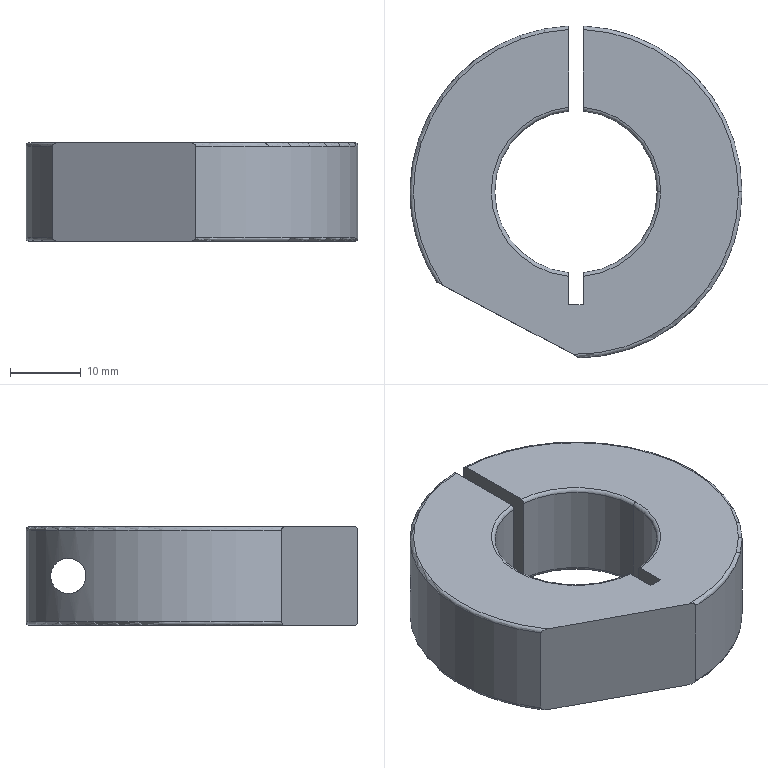Part | SolidWorks | features BaseBody 1 | 1 solid | 34 faces | box 47 x 46.973 x 14 mm | volume 15967 mm3 | cylinder 13 | torus 12 | plane 9 | commonest cylinder face diameters 11 x3 23 x3 47 x3 5 x2 6.4 x2
STEP:
#1=CARTESIAN_POINT('',(1.,17.5,-3.2));
#2=VERTEX_POINT('',#1);
#3=CARTESIAN_POINT('',(1.,17.5,3.2));
#4=VERTEX_POINT('',#3);
#5=CARTESIAN_POINT('',(1.,17.5,0.));
#6=DIRECTION('',(-1.,0.,0.));
#7=DIRECTION('',(0.,1.,0.));
#8=AXIS2_PLACEMENT_3D('',#5,#6,#7);
#9=CIRCLE('',#8,3.2);
#10=EDGE_CURVE('',#2,#4,#9,.T.);
#11=ORIENTED_EDGE('',*,*,#10,.T.);
#12=CARTESIAN_POINT('',(5.,17.5,3.2));
#13=VERTEX_POINT('',#12);
#14=CARTESIAN_POINT('',(5.,17.5,3.2));
#15=DIRECTION('',(1.,0.,0.));
#16=VECTOR('',#15,1000.);
#17=LINE('',#14,#16);
#18=EDGE_CURVE('',#4,#13,#17,.T.);
#19=ORIENTED_EDGE('',*,*,#18,.T.);
#20=CARTESIAN_POINT('',(5.,17.5,-3.2));
#21=VERTEX_POINT('',#20);
#22=CARTESIAN_POINT('',(5.,17.5,0.));
#23=DIRECTION('',(1.,0.,0.));
#24=DIRECTION('',(0.,0.,-1.));
#25=AXIS2_PLACEMENT_3D('',#22,#23,#24);
#26=CIRCLE('',#25,3.2);
#27=EDGE_CURVE('',#13,#21,#26,.T.);
#28=ORIENTED_EDGE('',*,*,#27,.T.);
#29=CARTESIAN_POINT('',(5.,17.5,-3.2));
#30=DIRECTION('',(1.,0.,0.));
#31=VECTOR('',#30,1000.);
#32=LINE('',#29,#31);
#33=EDGE_CURVE('',#2,#21,#32,.T.);
#34=ORIENTED_EDGE('',*,*,#33,.F.);
#35=EDGE_LOOP('',(#11,#19,#28,#34));
#36=FACE_OUTER_BOUND('',#35,.T.);
#37=CARTESIAN_POINT('',(5.,17.5,0.));
#38=DIRECTION('',(1.,0.,0.));
#39=DIRECTION('',(0.,0.,-1.));
#40=AXIS2_PLACEMENT_3D('',#37,#38,#39);
#41=CYLINDRICAL_SURFACE('',#40,3.2);
#42=ADVANCED_FACE('',(#36),#41,.F.);
#43=CARTESIAN_POINT('',(-15.684,17.5,2.5));
#44=VERTEX_POINT('',#43);
#45=CARTESIAN_POINT('',(-15.684,17.5,-2.5));
#46=VERTEX_POINT('',#45);
#47=CARTESIAN_POINT('',(-15.684,17.5,2.5));
#48=CARTESIAN_POINT('',(-15.98,17.235,2.5));
#49=CARTESIAN_POINT('',(-16.263,16.968,2.459));
#50=CARTESIAN_POINT('',(-16.67,16.565,2.323));
#51=CARTESIAN_POINT('',(-16.803,16.43,2.264));
#52=CARTESIAN_POINT('',(-17.059,16.164,2.118));
#53=CARTESIAN_POINT('',(-17.18,16.035,2.032));
#54=CARTESIAN_POINT('',(-17.409,15.787,1.828));
#55=CARTESIAN_POINT('',(-17.517,15.666,1.708));
#56=CARTESIAN_POINT('',(-17.709,15.449,1.44));
#57=CARTESIAN_POINT('',(-17.794,15.351,1.291));
#58=CARTESIAN_POINT('',(-17.937,15.183,0.9577));
#59=CARTESIAN_POINT('',(-17.993,15.117,0.7803));
#60=CARTESIAN_POINT('',(-18.07,15.025,0.4013));
#61=CARTESIAN_POINT('',(-18.09,15.,0.2036));
#62=CARTESIAN_POINT('',(-18.09,15.,-0.1912));
#63=CARTESIAN_POINT('',(-18.071,15.023,-0.3914));
#64=CARTESIAN_POINT('',(-17.996,15.113,-0.7689));
#65=CARTESIAN_POINT('',(-17.939,15.181,-0.951));
#66=CARTESIAN_POINT('',(-17.798,15.346,-1.282));
#67=CARTESIAN_POINT('',(-17.712,15.445,-1.435));
#68=CARTESIAN_POINT('',(-17.521,15.662,-1.704));
#69=CARTESIAN_POINT('',(-17.415,15.78,-1.821));
#70=CARTESIAN_POINT('',(-17.186,16.029,-2.028));
#71=CARTESIAN_POINT('',(-17.063,16.16,-2.116));
#72=CARTESIAN_POINT('',(-16.81,16.423,-2.261));
#73=CARTESIAN_POINT('',(-16.678,16.557,-2.32));
#74=CARTESIAN_POINT('',(-16.405,16.827,-2.412));
#75=CARTESIAN_POINT('',(-16.264,16.964,-2.446));
#76=CARTESIAN_POINT('',(-15.978,17.234,-2.49));
#77=CARTESIAN_POINT('',(-15.832,17.367,-2.5));
#78=CARTESIAN_POINT('',(-15.684,17.5,-2.5));
#79=B_SPLINE_CURVE_WITH_KNOTS('',3,(#47,#48,#49,#50,#51,#52,#53,#54,#55,#56,#57,#58,#59,#60,#61,#62,#63,#64,#65,#66,#67,#68,#69,#70,#71,#72,#73,#74,#75,#76,#77,#78),.UNSPECIFIED.,.F.,.F.,(4,2,2,2,2,2,2,2,2,2,2,2,2,2,2,4),(0.,0.001174,0.001761,0.002347,0.002934,0.003521,0.004108,0.004695,0.005282,0.005868,0.006455,0.007042,0.007629,0.008216,0.008803,0.009389),.UNSPECIFIED.);
#80=EDGE_CURVE('',#44,#46,#79,.T.);
#81=ORIENTED_EDGE('',*,*,#80,.F.);
#82=CARTESIAN_POINT('',(-1.,17.5,2.5));
#83=VERTEX_POINT('',#82);
#84=CARTESIAN_POINT('',(5.,17.5,2.5));
#85=DIRECTION('',(1.,0.,0.));
#86=VECTOR('',#85,1000.);
#87=LINE('',#84,#86);
#88=EDGE_CURVE('',#44,#83,#87,.T.);
#89=ORIENTED_EDGE('',*,*,#88,.T.);
#90=CARTESIAN_POINT('',(-1.,17.5,-2.5));
#91=VERTEX_POINT('',#90);
#92=CARTESIAN_POINT('',(-1.,17.5,0.));
#93=DIRECTION('',(1.,0.,0.));
#94=DIRECTION('',(0.,-1.,0.));
#95=AXIS2_PLACEMENT_3D('',#92,#93,#94);
#96=CIRCLE('',#95,2.5);
#97=EDGE_CURVE('',#83,#91,#96,.T.);
#98=ORIENTED_EDGE('',*,*,#97,.T.);
#99=CARTESIAN_POINT('',(5.,17.5,-2.5));
#100=DIRECTION('',(1.,0.,0.));
#101=VECTOR('',#100,1000.);
#102=LINE('',#99,#101);
#103=EDGE_CURVE('',#46,#91,#102,.T.);
#104=ORIENTED_EDGE('',*,*,#103,.F.);
#105=EDGE_LOOP('',(#81,#89,#98,#104));
#106=FACE_OUTER_BOUND('',#105,.T.);
#107=CARTESIAN_POINT('',(5.,17.5,0.));
#108=DIRECTION('',(1.,0.,0.));
#109=DIRECTION('',(0.,0.,-1.));
#110=AXIS2_PLACEMENT_3D('',#107,#108,#109);
#111=CYLINDRICAL_SURFACE('',#110,2.5);
#112=ADVANCED_FACE('',(#106),#111,.F.);
#113=CARTESIAN_POINT('',(5.,17.5,5.5));
#114=VERTEX_POINT('',#113);
#115=CARTESIAN_POINT('',(5.,17.5,-5.5));
#116=VERTEX_POINT('',#115);
#117=CARTESIAN_POINT('',(5.,17.5,0.));
#118=DIRECTION('',(1.,0.,0.));
#119=DIRECTION('',(0.,0.,-1.));
#120=AXIS2_PLACEMENT_3D('',#117,#118,#119);
#121=CIRCLE('',#120,5.5);
#122=EDGE_CURVE('',#114,#116,#121,.T.);
#123=ORIENTED_EDGE('',*,*,#122,.F.);
#124=CARTESIAN_POINT('',(15.684,17.5,5.5));
#125=VERTEX_POINT('',#124);
#126=CARTESIAN_POINT('',(5.,17.5,5.5));
#127=DIRECTION('',(1.,0.,0.));
#128=VECTOR('',#127,1000.);
#129=LINE('',#126,#128);
#130=EDGE_CURVE('',#114,#125,#129,.T.);
#131=ORIENTED_EDGE('',*,*,#130,.T.);
#132=CARTESIAN_POINT('',(15.684,17.5,-5.5));
#133=VERTEX_POINT('',#132);
#134=CARTESIAN_POINT('',(15.684,17.5,-5.5));
#135=CARTESIAN_POINT('',(16.311,16.938,-5.5));
#136=CARTESIAN_POINT('',(16.898,16.352,-5.417));
#137=CARTESIAN_POINT('',(17.717,15.445,-5.111));
#138=CARTESIAN_POINT('',(17.978,15.14,-4.979));
#139=CARTESIAN_POINT('',(18.462,14.545,-4.651));
#140=CARTESIAN_POINT('',(18.688,14.253,-4.454));
#141=CARTESIAN_POINT('',(19.105,13.689,-3.983));
#142=CARTESIAN_POINT('',(19.289,13.426,-3.715));
#143=CARTESIAN_POINT('',(19.613,12.948,-3.111));
#144=CARTESIAN_POINT('',(19.754,12.731,-2.769));
#145=CARTESIAN_POINT('',(19.976,12.379,-2.047));
#146=CARTESIAN_POINT('',(20.061,12.24,-1.662));
#147=CARTESIAN_POINT('',(20.176,12.049,-0.8451));
#148=CARTESIAN_POINT('',(20.205,12.001,-0.4313));
#149=CARTESIAN_POINT('',(20.205,12.,0.1975));
#150=CARTESIAN_POINT('',(20.199,12.011,0.41));
#151=CARTESIAN_POINT('',(20.17,12.059,0.8273));
#152=CARTESIAN_POINT('',(20.149,12.094,1.033));
#153=CARTESIAN_POINT('',(20.065,12.233,1.638));
#154=CARTESIAN_POINT('',(19.98,12.374,2.033));
#155=CARTESIAN_POINT('',(19.813,12.638,2.579));
#156=CARTESIAN_POINT('',(19.751,12.735,2.753));
#157=CARTESIAN_POINT('',(19.613,12.945,3.089));
#158=CARTESIAN_POINT('',(19.538,13.059,3.251));
#159=CARTESIAN_POINT('',(19.293,13.42,3.709));
#160=CARTESIAN_POINT('',(19.108,13.684,3.977));
#161=CARTESIAN_POINT('',(18.798,14.104,4.33));
#162=CARTESIAN_POINT('',(18.688,14.249,4.44));
#163=CARTESIAN_POINT('',(18.462,14.541,4.64));
#164=CARTESIAN_POINT('',(18.344,14.689,4.731));
#165=CARTESIAN_POINT('',(17.98,15.137,4.978));
#166=CARTESIAN_POINT('',(17.718,15.443,5.111));
#167=CARTESIAN_POINT('',(16.899,16.35,5.416));
#168=CARTESIAN_POINT('',(16.312,16.938,5.5));
#169=CARTESIAN_POINT('',(15.684,17.5,5.5));
#170=B_SPLINE_CURVE_WITH_KNOTS('',3,(#134,#135,#136,#137,#138,#139,#140,#141,#142,#143,#144,#145,#146,#147,#148,#149,#150,#151,#152,#153,#154,#155,#156,#157,#158,#159,#160,#161,#162,#163,#164,#165,#166,#167,#168,#169),.UNSPECIFIED.,.F.,.F.,(4,2,2,2,2,2,2,2,2,2,2,2,2,2,2,2,2,4),(0.,0.0025,0.00375,0.005,0.006249,0.007499,0.008749,0.009999,0.01062,0.01125,0.0125,0.01312,0.01375,0.015,0.01562,0.01625,0.0175,0.02),.UNSPECIFIED.);
#171=EDGE_CURVE('',#133,#125,#170,.T.);
#172=ORIENTED_EDGE('',*,*,#171,.F.);
#173=CARTESIAN_POINT('',(5.,17.5,-5.5));
#174=DIRECTION('',(1.,0.,0.));
#175=VECTOR('',#174,1000.);
#176=LINE('',#173,#175);
#177=EDGE_CURVE('',#116,#133,#176,.T.);
#178=ORIENTED_EDGE('',*,*,#177,.F.);
#179=EDGE_LOOP('',(#123,#131,#172,#178));
#180=FACE_OUTER_BOUND('',#179,.T.);
#181=CARTESIAN_POINT('',(5.,17.5,0.));
#182=DIRECTION('',(1.,0.,0.));
#183=DIRECTION('',(0.,0.,-1.));
#184=AXIS2_PLACEMENT_3D('',#181,#182,#183);
#185=CYLINDRICAL_SURFACE('',#184,5.5);
#186=ADVANCED_FACE('',(#180),#185,.F.);
#187=CARTESIAN_POINT('',(5.,22.962,-0.646));
#188=VERTEX_POINT('',#187);
#189=CARTESIAN_POINT('',(5.,17.5,0.));
#190=DIRECTION('',(1.,0.,0.));
#191=DIRECTION('',(0.,0.,-1.));
#192=AXIS2_PLACEMENT_3D('',#189,#190,#191);
#193=CIRCLE('',#192,5.5);
#194=EDGE_CURVE('',#116,#188,#193,.T.);
#195=ORIENTED_EDGE('',*,*,#194,.F.);
#196=ORIENTED_EDGE('',*,*,#177,.T.);
#197=CARTESIAN_POINT('',(5.,22.962,-0.646));
#198=CARTESIAN_POINT('',(5.136,22.932,-0.8973));
#199=CARTESIAN_POINT('',(5.317,22.891,-1.106));
#200=CARTESIAN_POINT('',(5.709,22.797,-1.494));
#201=CARTESIAN_POINT('',(5.922,22.743,-1.672));
#202=CARTESIAN_POINT('',(6.577,22.565,-2.172));
#203=CARTESIAN_POINT('',(7.033,22.428,-2.462));
#204=CARTESIAN_POINT('',(7.954,22.118,-3.003));
#205=CARTESIAN_POINT('',(8.422,21.945,-3.253));
#206=CARTESIAN_POINT('',(9.361,21.561,-3.722));
#207=CARTESIAN_POINT('',(9.834,21.35,-3.94));
#208=CARTESIAN_POINT('',(11.235,20.667,-4.537));
#209=CARTESIAN_POINT('',(12.152,20.143,-4.867));
#210=CARTESIAN_POINT('',(13.504,19.24,-5.227));
#211=CARTESIAN_POINT('',(13.952,18.919,-5.325));
#212=CARTESIAN_POINT('',(14.834,18.235,-5.462));
#213=CARTESIAN_POINT('',(15.265,17.876,-5.5));
#214=CARTESIAN_POINT('',(15.684,17.5,-5.5));
#215=B_SPLINE_CURVE_WITH_KNOTS('',3,(#197,#198,#199,#200,#201,#202,#203,#204,#205,#206,#207,#208,#209,#210,#211,#212,#213,#214),.UNSPECIFIED.,.F.,.F.,(4,2,2,2,2,2,2,2,4),(-0.01338,-0.01255,-0.01171,-0.01004,-0.008365,-0.006692,-0.003346,-0.001673,0.),.UNSPECIFIED.);
#216=EDGE_CURVE('',#188,#133,#215,.T.);
#217=ORIENTED_EDGE('',*,*,#216,.F.);
#218=EDGE_LOOP('',(#195,#196,#217));
#219=FACE_OUTER_BOUND('',#218,.T.);
#220=CARTESIAN_POINT('',(5.,17.5,0.));
#221=DIRECTION('',(1.,0.,0.));
#222=DIRECTION('',(0.,0.,-1.));
#223=AXIS2_PLACEMENT_3D('',#220,#221,#222);
#224=CYLINDRICAL_SURFACE('',#223,5.5);
#225=ADVANCED_FACE('',(#219),#224,.F.);
#226=CARTESIAN_POINT('',(0.5201,-23.494,-6.5));
#227=VERTEX_POINT('',#226);
#228=CARTESIAN_POINT('',(23.5,0.,-6.5));
#229=VERTEX_POINT('',#228);
#230=CARTESIAN_POINT('',(0.,0.,-6.5));
#231=DIRECTION('',(0.,0.,1.));
#232=DIRECTION('',(1.,0.,0.));
#233=AXIS2_PLACEMENT_3D('',#230,#231,#232);
#234=CIRCLE('',#233,23.5);
#235=EDGE_CURVE('',#227,#229,#234,.T.);
#236=ORIENTED_EDGE('',*,*,#235,.T.);
#237=CARTESIAN_POINT('',(23.5,0.,6.5));
#238=VERTEX_POINT('',#237);
#239=CARTESIAN_POINT('',(23.5,0.,0.));
#240=DIRECTION('',(0.,0.,1.));
#241=VECTOR('',#240,1000.);
#242=LINE('',#239,#241);
#243=EDGE_CURVE('',#229,#238,#242,.T.);
#244=ORIENTED_EDGE('',*,*,#243,.T.);
#245=CARTESIAN_POINT('',(0.5201,-23.494,6.5));
#246=VERTEX_POINT('',#245);
#247=CARTESIAN_POINT('',(0.,0.,6.5));
#248=DIRECTION('',(0.,0.,1.));
#249=DIRECTION('',(1.,0.,0.));
#250=AXIS2_PLACEMENT_3D('',#247,#248,#249);
#251=CIRCLE('',#250,23.5);
#252=EDGE_CURVE('',#246,#238,#251,.T.);
#253=ORIENTED_EDGE('',*,*,#252,.F.);
#254=CARTESIAN_POINT('',(0.5201,-23.494,0.));
#255=DIRECTION('',(0.,0.,-1.));
#256=VECTOR('',#255,1000.);
#257=LINE('',#254,#256);
#258=EDGE_CURVE('',#246,#227,#257,.T.);
#259=ORIENTED_EDGE('',*,*,#258,.T.);
#260=EDGE_LOOP('',(#236,#244,#253,#259));
#261=FACE_OUTER_BOUND('',#260,.T.);
#262=CARTESIAN_POINT('',(0.,0.,0.));
#263=DIRECTION('',(0.,0.,1.));
#264=DIRECTION('',(1.,0.,0.));
#265=AXIS2_PLACEMENT_3D('',#262,#263,#264);
#266=CYLINDRICAL_SURFACE('',#265,23.5);
#267=ADVANCED_FACE('',(#261),#266,.T.);
#268=CARTESIAN_POINT('',(1.,-11.456,-6.5));
#269=VERTEX_POINT('',#268);
#270=CARTESIAN_POINT('',(11.5,0.,-6.5));
#271=VERTEX_POINT('',#270);
#272=CARTESIAN_POINT('',(0.,0.,-6.5));
#273=DIRECTION('',(0.,0.,1.));
#274=DIRECTION('',(1.,0.,0.));
#275=AXIS2_PLACEMENT_3D('',#272,#273,#274);
#276=CIRCLE('',#275,11.5);
#277=EDGE_CURVE('',#269,#271,#276,.T.);
#278=ORIENTED_EDGE('',*,*,#277,.T.);
#279=CARTESIAN_POINT('',(12.,0.,-7.));
#280=VERTEX_POINT('',#279);
#281=CARTESIAN_POINT('',(12.,0.,-6.5));
#282=DIRECTION('',(0.,-1.,0.));
#283=DIRECTION('',(0.,0.,-1.));
#284=AXIS2_PLACEMENT_3D('',#281,#282,#283);
#285=CIRCLE('',#284,0.5);
#286=EDGE_CURVE('',#271,#280,#285,.T.);
#287=ORIENTED_EDGE('',*,*,#286,.T.);
#288=CARTESIAN_POINT('',(1.,-11.958,-7.));
#289=VERTEX_POINT('',#288);
#290=CARTESIAN_POINT('',(0.,0.,-7.));
#291=DIRECTION('',(0.,0.,1.));
#292=DIRECTION('',(1.,0.,0.));
#293=AXIS2_PLACEMENT_3D('',#290,#291,#292);
#294=CIRCLE('',#293,12.);
#295=EDGE_CURVE('',#289,#280,#294,.T.);
#296=ORIENTED_EDGE('',*,*,#295,.F.);
#297=CARTESIAN_POINT('',(1.,-11.958,-7.));
#298=CARTESIAN_POINT('',(1.,-11.826,-7.));
#299=CARTESIAN_POINT('',(1.,-11.697,-6.946));
#300=CARTESIAN_POINT('',(1.,-11.511,-6.762));
#301=CARTESIAN_POINT('',(1.,-11.456,-6.632));
#302=CARTESIAN_POINT('',(1.,-11.456,-6.5));
#303=B_SPLINE_CURVE_WITH_KNOTS('',3,(#297,#298,#299,#300,#301,#302),.UNSPECIFIED.,.F.,.F.,(4,2,4),(0.,0.0003912,0.0007825),.UNSPECIFIED.);
#304=EDGE_CURVE('',#289,#269,#303,.T.);
#305=ORIENTED_EDGE('',*,*,#304,.T.);
#306=EDGE_LOOP('',(#278,#287,#296,#305));
#307=FACE_OUTER_BOUND('',#306,.T.);
#308=CARTESIAN_POINT('',(0.,0.,-6.5));
#309=DIRECTION('',(0.,0.,1.));
#310=DIRECTION('',(1.,0.,0.));
#311=AXIS2_PLACEMENT_3D('',#308,#309,#310);
#312=TOROIDAL_SURFACE('',#311,12.,0.5);
#313=ADVANCED_FACE('',(#307),#312,.T.);
#314=CARTESIAN_POINT('',(1.,11.456,-6.5));
#315=VERTEX_POINT('',#314);
#316=CARTESIAN_POINT('',(0.,0.,-6.5));
#317=DIRECTION('',(0.,0.,1.));
#318=DIRECTION('',(1.,0.,0.));
#319=AXIS2_PLACEMENT_3D('',#316,#317,#318);
#320=CIRCLE('',#319,11.5);
#321=EDGE_CURVE('',#271,#315,#320,.T.);
#322=ORIENTED_EDGE('',*,*,#321,.F.);
#323=CARTESIAN_POINT('',(11.5,0.,6.5));
#324=VERTEX_POINT('',#323);
#325=CARTESIAN_POINT('',(11.5,0.,0.));
#326=DIRECTION('',(0.,0.,1.));
#327=VECTOR('',#326,1000.);
#328=LINE('',#325,#327);
#329=EDGE_CURVE('',#271,#324,#328,.T.);
#330=ORIENTED_EDGE('',*,*,#329,.T.);
#331=CARTESIAN_POINT('',(1.,11.456,6.5));
#332=VERTEX_POINT('',#331);
#333=CARTESIAN_POINT('',(0.,0.,6.5));
#334=DIRECTION('',(0.,0.,1.));
#335=DIRECTION('',(1.,0.,0.));
#336=AXIS2_PLACEMENT_3D('',#333,#334,#335);
#337=CIRCLE('',#336,11.5);
#338=EDGE_CURVE('',#324,#332,#337,.T.);
#339=ORIENTED_EDGE('',*,*,#338,.T.);
#340=CARTESIAN_POINT('',(1.,11.456,0.));
#341=DIRECTION('',(0.,0.,-1.));
#342=VECTOR('',#341,1000.);
#343=LINE('',#340,#342);
#344=EDGE_CURVE('',#332,#315,#343,.T.);
#345=ORIENTED_EDGE('',*,*,#344,.T.);
#346=EDGE_LOOP('',(#322,#330,#339,#345));
#347=FACE_OUTER_BOUND('',#346,.T.);
#348=CARTESIAN_POINT('',(0.,0.,0.));
#349=DIRECTION('',(0.,0.,1.));
#350=DIRECTION('',(1.,0.,0.));
#351=AXIS2_PLACEMENT_3D('',#348,#349,#350);
#352=CYLINDRICAL_SURFACE('',#351,11.5);
#353=ADVANCED_FACE('',(#347),#352,.F.);
#354=CARTESIAN_POINT('',(1.,-11.958,7.));
#355=VERTEX_POINT('',#354);
#356=CARTESIAN_POINT('',(12.,0.,7.));
#357=VERTEX_POINT('',#356);
#358=CARTESIAN_POINT('',(0.,0.,7.));
#359=DIRECTION('',(0.,0.,1.));
#360=DIRECTION('',(1.,0.,0.));
#361=AXIS2_PLACEMENT_3D('',#358,#359,#360);
#362=CIRCLE('',#361,12.);
#363=EDGE_CURVE('',#355,#357,#362,.T.);
#364=ORIENTED_EDGE('',*,*,#363,.T.);
#365=CARTESIAN_POINT('',(12.,0.,6.5));
#366=DIRECTION('',(0.,-1.,0.));
#367=DIRECTION('',(0.,0.,-1.));
#368=AXIS2_PLACEMENT_3D('',#365,#366,#367);
#369=CIRCLE('',#368,0.5);
#370=EDGE_CURVE('',#357,#324,#369,.T.);
#371=ORIENTED_EDGE('',*,*,#370,.T.);
#372=CARTESIAN_POINT('',(1.,-11.456,6.5));
#373=VERTEX_POINT('',#372);
#374=CARTESIAN_POINT('',(0.,0.,6.5));
#375=DIRECTION('',(0.,0.,1.));
#376=DIRECTION('',(1.,0.,0.));
#377=AXIS2_PLACEMENT_3D('',#374,#375,#376);
#378=CIRCLE('',#377,11.5);
#379=EDGE_CURVE('',#373,#324,#378,.T.);
#380=ORIENTED_EDGE('',*,*,#379,.F.);
#381=CARTESIAN_POINT('',(1.,-11.456,6.5));
#382=CARTESIAN_POINT('',(1.,-11.456,6.632));
#383=CARTESIAN_POINT('',(1.,-11.511,6.762));
#384=CARTESIAN_POINT('',(1.,-11.696,6.946));
#385=CARTESIAN_POINT('',(1.,-11.826,7.));
#386=CARTESIAN_POINT('',(1.,-11.958,7.));
#387=B_SPLINE_CURVE_WITH_KNOTS('',3,(#381,#382,#383,#384,#385,#386),.UNSPECIFIED.,.F.,.F.,(4,2,4),(0.,0.0003912,0.0007825),.UNSPECIFIED.);
#388=EDGE_CURVE('',#373,#355,#387,.T.);
#389=ORIENTED_EDGE('',*,*,#388,.T.);
#390=EDGE_LOOP('',(#364,#371,#380,#389));
#391=FACE_OUTER_BOUND('',#390,.T.);
#392=CARTESIAN_POINT('',(0.,0.,6.5));
#393=DIRECTION('',(0.,0.,1.));
#394=DIRECTION('',(1.,0.,0.));
#395=AXIS2_PLACEMENT_3D('',#392,#393,#394);
#396=TOROIDAL_SURFACE('',#395,12.,0.5);
#397=ADVANCED_FACE('',(#391),#396,.T.);
#398=ORIENTED_EDGE('',*,*,#252,.T.);
#399=CARTESIAN_POINT('',(23.,0.,7.));
#400=VERTEX_POINT('',#399);
#401=CARTESIAN_POINT('',(23.,0.,6.5));
#402=DIRECTION('',(0.,-1.,0.));
#403=DIRECTION('',(0.,0.,-1.));
#404=AXIS2_PLACEMENT_3D('',#401,#402,#403);
#405=CIRCLE('',#404,0.5);
#406=EDGE_CURVE('',#238,#400,#405,.T.);
#407=ORIENTED_EDGE('',*,*,#406,.T.);
#408=CARTESIAN_POINT('',(-0.4165,-22.996,7.));
#409=VERTEX_POINT('',#408);
#410=CARTESIAN_POINT('',(0.,0.,7.));
#411=DIRECTION('',(0.,0.,1.));
#412=DIRECTION('',(1.,0.,0.));
#413=AXIS2_PLACEMENT_3D('',#410,#411,#412);
#414=CIRCLE('',#413,23.);
#415=EDGE_CURVE('',#409,#400,#414,.T.);
#416=ORIENTED_EDGE('',*,*,#415,.F.);
#417=CARTESIAN_POINT('',(-0.4165,-22.996,7.));
#418=CARTESIAN_POINT('',(-0.2296,-23.096,7.));
#419=CARTESIAN_POINT('',(-0.04627,-23.193,6.976));
#420=CARTESIAN_POINT('',(0.219,-23.334,6.876));
#421=CARTESIAN_POINT('',(0.307,-23.381,6.831));
#422=CARTESIAN_POINT('',(0.4183,-23.44,6.733));
#423=CARTESIAN_POINT('',(0.4524,-23.458,6.695));
#424=CARTESIAN_POINT('',(0.5036,-23.485,6.606));
#425=CARTESIAN_POINT('',(0.5201,-23.494,6.554));
#426=CARTESIAN_POINT('',(0.5201,-23.494,6.5));
#427=B_SPLINE_CURVE_WITH_KNOTS('',3,(#417,#418,#419,#420,#421,#422,#423,#424,#425,#426),.UNSPECIFIED.,.F.,.F.,(4,2,2,2,4),(0.,0.0006261,0.0009391,0.001096,0.001252),.UNSPECIFIED.);
#428=EDGE_CURVE('',#409,#246,#427,.T.);
#429=ORIENTED_EDGE('',*,*,#428,.T.);
#430=EDGE_LOOP('',(#398,#407,#416,#429));
#431=FACE_OUTER_BOUND('',#430,.T.);
#432=CARTESIAN_POINT('',(0.,0.,6.5));
#433=DIRECTION('',(0.,0.,1.));
#434=DIRECTION('',(1.,0.,0.));
#435=AXIS2_PLACEMENT_3D('',#432,#433,#434);
#436=TOROIDAL_SURFACE('',#435,23.,0.5);
#437=ADVANCED_FACE('',(#431),#436,.T.);
#438=CARTESIAN_POINT('',(-0.4165,-22.996,-7.));
#439=VERTEX_POINT('',#438);
#440=CARTESIAN_POINT('',(23.,0.,-7.));
#441=VERTEX_POINT('',#440);
#442=CARTESIAN_POINT('',(0.,0.,-7.));
#443=DIRECTION('',(0.,0.,1.));
#444=DIRECTION('',(1.,0.,0.));
#445=AXIS2_PLACEMENT_3D('',#442,#443,#444);
#446=CIRCLE('',#445,23.);
#447=EDGE_CURVE('',#439,#441,#446,.T.);
#448=ORIENTED_EDGE('',*,*,#447,.T.);
#449=CARTESIAN_POINT('',(23.,0.,-6.5));
#450=DIRECTION('',(0.,-1.,0.));
#451=DIRECTION('',(0.,0.,-1.));
#452=AXIS2_PLACEMENT_3D('',#449,#450,#451);
#453=CIRCLE('',#452,0.5);
#454=EDGE_CURVE('',#441,#229,#453,.T.);
#455=ORIENTED_EDGE('',*,*,#454,.T.);
#456=ORIENTED_EDGE('',*,*,#235,.F.);
#457=CARTESIAN_POINT('',(0.5201,-23.494,-6.5));
#458=CARTESIAN_POINT('',(0.5201,-23.494,-6.554));
#459=CARTESIAN_POINT('',(0.5038,-23.486,-6.606));
#460=CARTESIAN_POINT('',(0.4528,-23.458,-6.695));
#461=CARTESIAN_POINT('',(0.4189,-23.44,-6.733));
#462=CARTESIAN_POINT('',(0.3077,-23.381,-6.83));
#463=CARTESIAN_POINT('',(0.2217,-23.336,-6.874));
#464=CARTESIAN_POINT('',(-0.04424,-23.194,-6.976));
#465=CARTESIAN_POINT('',(-0.2296,-23.096,-7.));
#466=CARTESIAN_POINT('',(-0.4165,-22.996,-7.));
#467=B_SPLINE_CURVE_WITH_KNOTS('',3,(#457,#458,#459,#460,#461,#462,#463,#464,#465,#466),.UNSPECIFIED.,.F.,.F.,(4,2,2,2,4),(0.,0.0001592,0.0003184,0.0006368,0.001274),.UNSPECIFIED.);
#468=EDGE_CURVE('',#227,#439,#467,.T.);
#469=ORIENTED_EDGE('',*,*,#468,.T.);
#470=EDGE_LOOP('',(#448,#455,#456,#469));
#471=FACE_OUTER_BOUND('',#470,.T.);
#472=CARTESIAN_POINT('',(0.,0.,-6.5));
#473=DIRECTION('',(0.,0.,1.));
#474=DIRECTION('',(1.,0.,0.));
#475=AXIS2_PLACEMENT_3D('',#472,#473,#474);
#476=TOROIDAL_SURFACE('',#475,23.,0.5);
#477=ADVANCED_FACE('',(#471),#476,.T.);
#478=CARTESIAN_POINT('',(-18.832,-13.205,7.));
#479=VERTEX_POINT('',#478);
#480=CARTESIAN_POINT('',(-14.598,-15.456,7.));
#481=DIRECTION('',(0.8829,-0.4695,0.));
#482=VECTOR('',#481,1000.);
#483=LINE('',#480,#482);
#484=EDGE_CURVE('',#479,#409,#483,.T.);
#485=ORIENTED_EDGE('',*,*,#484,.F.);
#486=CARTESIAN_POINT('',(-19.768,-12.707,6.5));
#487=VERTEX_POINT('',#486);
#488=CARTESIAN_POINT('',(-19.768,-12.707,6.5));
#489=CARTESIAN_POINT('',(-19.768,-12.707,6.554));
#490=CARTESIAN_POINT('',(-19.752,-12.715,6.606));
#491=CARTESIAN_POINT('',(-19.701,-12.742,6.695));
#492=CARTESIAN_POINT('',(-19.667,-12.76,6.733));
#493=CARTESIAN_POINT('',(-19.556,-12.82,6.83));
#494=CARTESIAN_POINT('',(-19.47,-12.865,6.874));
#495=CARTESIAN_POINT('',(-19.204,-13.007,6.976));
#496=CARTESIAN_POINT('',(-19.019,-13.105,7.));
#497=CARTESIAN_POINT('',(-18.832,-13.205,7.));
#498=B_SPLINE_CURVE_WITH_KNOTS('',3,(#488,#489,#490,#491,#492,#493,#494,#495,#496,#497),.UNSPECIFIED.,.F.,.F.,(4,2,2,2,4),(0.,0.0001592,0.0003184,0.0006368,0.001274),.UNSPECIFIED.);
#499=EDGE_CURVE('',#487,#479,#498,.T.);
#500=ORIENTED_EDGE('',*,*,#499,.F.);
#501=CARTESIAN_POINT('',(-19.768,-12.707,-6.5));
#502=VERTEX_POINT('',#501);
#503=CARTESIAN_POINT('',(-19.768,-12.707,0.));
#504=DIRECTION('',(0.,0.,1.));
#505=VECTOR('',#504,1000.);
#506=LINE('',#503,#505);
#507=EDGE_CURVE('',#502,#487,#506,.T.);
#508=ORIENTED_EDGE('',*,*,#507,.F.);
#509=CARTESIAN_POINT('',(-18.832,-13.205,-7.));
#510=VERTEX_POINT('',#509);
#511=CARTESIAN_POINT('',(-18.832,-13.205,-7.));
#512=CARTESIAN_POINT('',(-19.019,-13.105,-7.));
#513=CARTESIAN_POINT('',(-19.202,-13.008,-6.976));
#514=CARTESIAN_POINT('',(-19.467,-12.867,-6.876));
#515=CARTESIAN_POINT('',(-19.555,-12.82,-6.831));
#516=CARTESIAN_POINT('',(-19.667,-12.761,-6.733));
#517=CARTESIAN_POINT('',(-19.701,-12.743,-6.695));
#518=CARTESIAN_POINT('',(-19.752,-12.715,-6.606));
#519=CARTESIAN_POINT('',(-19.768,-12.707,-6.554));
#520=CARTESIAN_POINT('',(-19.768,-12.707,-6.5));
#521=B_SPLINE_CURVE_WITH_KNOTS('',3,(#511,#512,#513,#514,#515,#516,#517,#518,#519,#520),.UNSPECIFIED.,.F.,.F.,(4,2,2,2,4),(0.,0.0006261,0.0009391,0.001096,0.001252),.UNSPECIFIED.);
#522=EDGE_CURVE('',#510,#502,#521,.T.);
#523=ORIENTED_EDGE('',*,*,#522,.F.);
#524=CARTESIAN_POINT('',(-14.598,-15.456,-7.));
#525=DIRECTION('',(-0.8829,0.4695,0.));
#526=VECTOR('',#525,1000.);
#527=LINE('',#524,#526);
#528=EDGE_CURVE('',#439,#510,#527,.T.);
#529=ORIENTED_EDGE('',*,*,#528,.F.);
#530=ORIENTED_EDGE('',*,*,#468,.F.);
#531=ORIENTED_EDGE('',*,*,#258,.F.);
#532=ORIENTED_EDGE('',*,*,#428,.F.);
#533=EDGE_LOOP('',(#485,#500,#508,#523,#529,#530,#531,#532));
#534=FACE_OUTER_BOUND('',#533,.T.);
#535=CARTESIAN_POINT('',(6.662,-26.76,-108.789));
#536=DIRECTION('',(0.4695,0.8829,0.));
#537=DIRECTION('',(0.,0.,-1.));
#538=AXIS2_PLACEMENT_3D('',#535,#536,#537);
#539=PLANE('',#538);
#540=ADVANCED_FACE('',(#534),#539,.F.);
#541=CARTESIAN_POINT('',(1.,-16.,-7.));
#542=VERTEX_POINT('',#541);
#543=CARTESIAN_POINT('',(-1.,-16.,-7.));
#544=VERTEX_POINT('',#543);
#545=CARTESIAN_POINT('',(1.,-16.,-7.));
#546=DIRECTION('',(-1.,0.,0.));
#547=VECTOR('',#546,1000.);
#548=LINE('',#545,#547);
#549=EDGE_CURVE('',#542,#544,#548,.T.);
#550=ORIENTED_EDGE('',*,*,#549,.T.);
#551=CARTESIAN_POINT('',(-1.,-16.,7.));
#552=VERTEX_POINT('',#551);
#553=CARTESIAN_POINT('',(-1.,-16.,7.));
#554=DIRECTION('',(0.,0.,-1.));
#555=VECTOR('',#554,1000.);
#556=LINE('',#553,#555);
#557=EDGE_CURVE('',#552,#544,#556,.T.);
#558=ORIENTED_EDGE('',*,*,#557,.F.);
#559=CARTESIAN_POINT('',(1.,-16.,7.));
#560=VERTEX_POINT('',#559);
#561=CARTESIAN_POINT('',(1.,-16.,7.));
#562=DIRECTION('',(-1.,0.,0.));
#563=VECTOR('',#562,1000.);
#564=LINE('',#561,#563);
#565=EDGE_CURVE('',#560,#552,#564,.T.);
#566=ORIENTED_EDGE('',*,*,#565,.F.);
#567=CARTESIAN_POINT('',(1.,-16.,7.));
#568=DIRECTION('',(0.,0.,-1.));
#569=VECTOR('',#568,1000.);
#570=LINE('',#567,#569);
#571=EDGE_CURVE('',#560,#542,#570,.T.);
#572=ORIENTED_EDGE('',*,*,#571,.T.);
#573=EDGE_LOOP('',(#550,#558,#566,#572));
#574=FACE_OUTER_BOUND('',#573,.T.);
#575=CARTESIAN_POINT('',(1.,-16.,7.));
#576=DIRECTION('',(0.,-1.,0.));
#577=DIRECTION('',(0.,0.,-1.));
#578=AXIS2_PLACEMENT_3D('',#575,#576,#577);
#579=PLANE('',#578);
#580=ADVANCED_FACE('',(#574),#579,.F.);
#581=CARTESIAN_POINT('',(1.,-11.456,0.));
#582=DIRECTION('',(0.,0.,1.));
#583=VECTOR('',#582,1000.);
#584=LINE('',#581,#583);
#585=EDGE_CURVE('',#269,#373,#584,.T.);
#586=ORIENTED_EDGE('',*,*,#585,.F.);
#587=ORIENTED_EDGE('',*,*,#304,.F.);
#588=CARTESIAN_POINT('',(1.,29.175,-7.));
#589=DIRECTION('',(0.,-1.,0.));
#590=VECTOR('',#589,1000.);
#591=LINE('',#588,#590);
#592=EDGE_CURVE('',#289,#542,#591,.T.);
#593=ORIENTED_EDGE('',*,*,#592,.T.);
#594=ORIENTED_EDGE('',*,*,#571,.F.);
#595=CARTESIAN_POINT('',(1.,29.175,7.));
#596=DIRECTION('',(0.,-1.,0.));
#597=VECTOR('',#596,1000.);
#598=LINE('',#595,#597);
#599=EDGE_CURVE('',#355,#560,#598,.T.);
#600=ORIENTED_EDGE('',*,*,#599,.F.);
#601=ORIENTED_EDGE('',*,*,#388,.F.);
#602=EDGE_LOOP('',(#586,#587,#593,#594,#600,#601));
#603=FACE_OUTER_BOUND('',#602,.T.);
#604=CARTESIAN_POINT('',(1.,29.175,7.));
#605=DIRECTION('',(1.,0.,0.));
#606=DIRECTION('',(0.,-1.,0.));
#607=AXIS2_PLACEMENT_3D('',#604,#605,#606);
#608=PLANE('',#607);
#609=ADVANCED_FACE('',(#603),#608,.F.);
#610=CARTESIAN_POINT('',(-1.,-11.958,7.));
#611=VERTEX_POINT('',#610);
#612=CARTESIAN_POINT('',(-1.,29.175,7.));
#613=DIRECTION('',(0.,1.,0.));
#614=VECTOR('',#613,1000.);
#615=LINE('',#612,#614);
#616=EDGE_CURVE('',#552,#611,#615,.T.);
#617=ORIENTED_EDGE('',*,*,#616,.F.);
#618=ORIENTED_EDGE('',*,*,#557,.T.);
#619=CARTESIAN_POINT('',(-1.,-11.958,-7.));
#620=VERTEX_POINT('',#619);
#621=CARTESIAN_POINT('',(-1.,29.175,-7.));
#622=DIRECTION('',(0.,1.,0.));
#623=VECTOR('',#622,1000.);
#624=LINE('',#621,#623);
#625=EDGE_CURVE('',#544,#620,#624,.T.);
#626=ORIENTED_EDGE('',*,*,#625,.T.);
#627=CARTESIAN_POINT('',(-1.,-11.456,-6.5));
#628=VERTEX_POINT('',#627);
#629=CARTESIAN_POINT('',(-1.,-11.456,-6.5));
#630=CARTESIAN_POINT('',(-1.,-11.456,-6.632));
#631=CARTESIAN_POINT('',(-1.,-11.511,-6.762));
#632=CARTESIAN_POINT('',(-1.,-11.696,-6.946));
#633=CARTESIAN_POINT('',(-1.,-11.826,-7.));
#634=CARTESIAN_POINT('',(-1.,-11.958,-7.));
#635=B_SPLINE_CURVE_WITH_KNOTS('',3,(#629,#630,#631,#632,#633,#634),.UNSPECIFIED.,.F.,.F.,(4,2,4),(0.,0.0003912,0.0007825),.UNSPECIFIED.);
#636=EDGE_CURVE('',#628,#620,#635,.T.);
#637=ORIENTED_EDGE('',*,*,#636,.F.);
#638=CARTESIAN_POINT('',(-1.,-11.456,6.5));
#639=VERTEX_POINT('',#638);
#640=CARTESIAN_POINT('',(-1.,-11.456,0.));
#641=DIRECTION('',(0.,0.,-1.));
#642=VECTOR('',#641,1000.);
#643=LINE('',#640,#642);
#644=EDGE_CURVE('',#639,#628,#643,.T.);
#645=ORIENTED_EDGE('',*,*,#644,.F.);
#646=CARTESIAN_POINT('',(-1.,-11.958,7.));
#647=CARTESIAN_POINT('',(-1.,-11.826,7.));
#648=CARTESIAN_POINT('',(-1.,-11.697,6.946));
#649=CARTESIAN_POINT('',(-1.,-11.511,6.762));
#650=CARTESIAN_POINT('',(-1.,-11.456,6.632));
#651=CARTESIAN_POINT('',(-1.,-11.456,6.5));
#652=B_SPLINE_CURVE_WITH_KNOTS('',3,(#646,#647,#648,#649,#650,#651),.UNSPECIFIED.,.F.,.F.,(4,2,4),(0.,0.0003912,0.0007825),.UNSPECIFIED.);
#653=EDGE_CURVE('',#611,#639,#652,.T.);
#654=ORIENTED_EDGE('',*,*,#653,.F.);
#655=EDGE_LOOP('',(#617,#618,#626,#637,#645,#654));
#656=FACE_OUTER_BOUND('',#655,.T.);
#657=CARTESIAN_POINT('',(-1.,29.175,7.));
#658=DIRECTION('',(-1.,0.,0.));
#659=DIRECTION('',(0.,0.,1.));
#660=AXIS2_PLACEMENT_3D('',#657,#658,#659);
#661=PLANE('',#660);
#662=ADVANCED_FACE('',(#656),#661,.F.);
#663=CARTESIAN_POINT('',(-1.,17.5,0.));
#664=DIRECTION('',(1.,0.,0.));
#665=DIRECTION('',(0.,-1.,0.));
#666=AXIS2_PLACEMENT_3D('',#663,#664,#665);
#667=CIRCLE('',#666,2.5);
#668=EDGE_CURVE('',#91,#83,#667,.T.);
#669=ORIENTED_EDGE('',*,*,#668,.F.);
#670=ORIENTED_EDGE('',*,*,#97,.F.);
#671=EDGE_LOOP('',(#669,#670));
#672=FACE_BOUND('',#671,.T.);
#673=CARTESIAN_POINT('',(-1.,23.479,6.5));
#674=VERTEX_POINT('',#673);
#675=CARTESIAN_POINT('',(-1.,23.479,-6.5));
#676=VERTEX_POINT('',#675);
#677=CARTESIAN_POINT('',(-1.,23.479,0.));
#678=DIRECTION('',(0.,0.,-1.));
#679=VECTOR('',#678,1000.);
#680=LINE('',#677,#679);
#681=EDGE_CURVE('',#674,#676,#680,.T.);
#682=ORIENTED_EDGE('',*,*,#681,.F.);
#683=CARTESIAN_POINT('',(-1.,22.978,7.));
#684=VERTEX_POINT('',#683);
#685=CARTESIAN_POINT('',(-1.,22.978,7.));
#686=CARTESIAN_POINT('',(-1.,23.11,7.));
#687=CARTESIAN_POINT('',(-1.,23.24,6.946));
#688=CARTESIAN_POINT('',(-1.,23.424,6.762));
#689=CARTESIAN_POINT('',(-1.,23.479,6.632));
#690=CARTESIAN_POINT('',(-1.,23.479,6.5));
#691=B_SPLINE_CURVE_WITH_KNOTS('',3,(#685,#686,#687,#688,#689,#690),.UNSPECIFIED.,.F.,.F.,(4,2,4),(0.,0.0003907,0.0007814),.UNSPECIFIED.);
#692=EDGE_CURVE('',#684,#674,#691,.T.);
#693=ORIENTED_EDGE('',*,*,#692,.F.);
#694=CARTESIAN_POINT('',(-1.,11.958,7.));
#695=VERTEX_POINT('',#694);
#696=CARTESIAN_POINT('',(-1.,29.175,7.));
#697=DIRECTION('',(0.,1.,0.));
#698=VECTOR('',#697,1000.);
#699=LINE('',#696,#698);
#700=EDGE_CURVE('',#695,#684,#699,.T.);
#701=ORIENTED_EDGE('',*,*,#700,.F.);
#702=CARTESIAN_POINT('',(-1.,11.456,6.5));
#703=VERTEX_POINT('',#702);
#704=CARTESIAN_POINT('',(-1.,11.456,6.5));
#705=CARTESIAN_POINT('',(-1.,11.456,6.632));
#706=CARTESIAN_POINT('',(-1.,11.511,6.762));
#707=CARTESIAN_POINT('',(-1.,11.696,6.946));
#708=CARTESIAN_POINT('',(-1.,11.826,7.));
#709=CARTESIAN_POINT('',(-1.,11.958,7.));
#710=B_SPLINE_CURVE_WITH_KNOTS('',3,(#704,#705,#706,#707,#708,#709),.UNSPECIFIED.,.F.,.F.,(4,2,4),(0.,0.0003912,0.0007825),.UNSPECIFIED.);
#711=EDGE_CURVE('',#703,#695,#710,.T.);
#712=ORIENTED_EDGE('',*,*,#711,.F.);
#713=CARTESIAN_POINT('',(-1.,11.456,-6.5));
#714=VERTEX_POINT('',#713);
#715=CARTESIAN_POINT('',(-1.,11.456,0.));
#716=DIRECTION('',(0.,0.,1.));
#717=VECTOR('',#716,1000.);
#718=LINE('',#715,#717);
#719=EDGE_CURVE('',#714,#703,#718,.T.);
#720=ORIENTED_EDGE('',*,*,#719,.F.);
#721=CARTESIAN_POINT('',(-1.,11.958,-7.));
#722=VERTEX_POINT('',#721);
#723=CARTESIAN_POINT('',(-1.,11.958,-7.));
#724=CARTESIAN_POINT('',(-1.,11.826,-7.));
#725=CARTESIAN_POINT('',(-1.,11.697,-6.946));
#726=CARTESIAN_POINT('',(-1.,11.511,-6.762));
#727=CARTESIAN_POINT('',(-1.,11.456,-6.632));
#728=CARTESIAN_POINT('',(-1.,11.456,-6.5));
#729=B_SPLINE_CURVE_WITH_KNOTS('',3,(#723,#724,#725,#726,#727,#728),.UNSPECIFIED.,.F.,.F.,(4,2,4),(0.,0.0003912,0.0007825),.UNSPECIFIED.);
#730=EDGE_CURVE('',#722,#714,#729,.T.);
#731=ORIENTED_EDGE('',*,*,#730,.F.);
#732=CARTESIAN_POINT('',(-1.,22.978,-7.));
#733=VERTEX_POINT('',#732);
#734=CARTESIAN_POINT('',(-1.,29.175,-7.));
#735=DIRECTION('',(0.,1.,0.));
#736=VECTOR('',#735,1000.);
#737=LINE('',#734,#736);
#738=EDGE_CURVE('',#722,#733,#737,.T.);
#739=ORIENTED_EDGE('',*,*,#738,.T.);
#740=CARTESIAN_POINT('',(-1.,23.479,-6.5));
#741=CARTESIAN_POINT('',(-1.,23.479,-6.632));
#742=CARTESIAN_POINT('',(-1.,23.424,-6.761));
#743=CARTESIAN_POINT('',(-1.,23.24,-6.946));
#744=CARTESIAN_POINT('',(-1.,23.11,-7.));
#745=CARTESIAN_POINT('',(-1.,22.978,-7.));
#746=B_SPLINE_CURVE_WITH_KNOTS('',3,(#740,#741,#742,#743,#744,#745),.UNSPECIFIED.,.F.,.F.,(4,2,4),(0.,0.0003907,0.0007814),.UNSPECIFIED.);
#747=EDGE_CURVE('',#676,#733,#746,.T.);
#748=ORIENTED_EDGE('',*,*,#747,.F.);
#749=EDGE_LOOP('',(#682,#693,#701,#712,#720,#731,#739,#748));
#750=FACE_OUTER_BOUND('',#749,.T.);
#751=CARTESIAN_POINT('',(-1.,29.175,7.));
#752=DIRECTION('',(-1.,0.,0.));
#753=DIRECTION('',(0.,0.,1.));
#754=AXIS2_PLACEMENT_3D('',#751,#752,#753);
#755=PLANE('',#754);
#756=ADVANCED_FACE('',(#672,#750),#755,.F.);
#757=ORIENTED_EDGE('',*,*,#10,.F.);
#758=CARTESIAN_POINT('',(1.,17.5,0.));
#759=DIRECTION('',(-1.,0.,0.));
#760=DIRECTION('',(0.,1.,0.));
#761=AXIS2_PLACEMENT_3D('',#758,#759,#760);
#762=CIRCLE('',#761,3.2);
#763=EDGE_CURVE('',#4,#2,#762,.T.);
#764=ORIENTED_EDGE('',*,*,#763,.F.);
#765=EDGE_LOOP('',(#757,#764));
#766=FACE_BOUND('',#765,.T.);
#767=CARTESIAN_POINT('',(1.,22.978,-7.));
#768=VERTEX_POINT('',#767);
#769=CARTESIAN_POINT('',(1.,11.958,-7.));
#770=VERTEX_POINT('',#769);
#771=CARTESIAN_POINT('',(1.,29.175,-7.));
#772=DIRECTION('',(0.,-1.,0.));
#773=VECTOR('',#772,1000.);
#774=LINE('',#771,#773);
#775=EDGE_CURVE('',#768,#770,#774,.T.);
#776=ORIENTED_EDGE('',*,*,#775,.T.);
#777=CARTESIAN_POINT('',(1.,11.456,-6.5));
#778=CARTESIAN_POINT('',(1.,11.456,-6.632));
#779=CARTESIAN_POINT('',(1.,11.511,-6.762));
#780=CARTESIAN_POINT('',(1.,11.696,-6.946));
#781=CARTESIAN_POINT('',(1.,11.826,-7.));
#782=CARTESIAN_POINT('',(1.,11.958,-7.));
#783=B_SPLINE_CURVE_WITH_KNOTS('',3,(#777,#778,#779,#780,#781,#782),.UNSPECIFIED.,.F.,.F.,(4,2,4),(0.,0.0003912,0.0007825),.UNSPECIFIED.);
#784=EDGE_CURVE('',#315,#770,#783,.T.);
#785=ORIENTED_EDGE('',*,*,#784,.F.);
#786=ORIENTED_EDGE('',*,*,#344,.F.);
#787=CARTESIAN_POINT('',(1.,11.958,7.));
#788=VERTEX_POINT('',#787);
#789=CARTESIAN_POINT('',(1.,11.958,7.));
#790=CARTESIAN_POINT('',(1.,11.826,7.));
#791=CARTESIAN_POINT('',(1.,11.697,6.946));
#792=CARTESIAN_POINT('',(1.,11.511,6.762));
#793=CARTESIAN_POINT('',(1.,11.456,6.632));
#794=CARTESIAN_POINT('',(1.,11.456,6.5));
#795=B_SPLINE_CURVE_WITH_KNOTS('',3,(#789,#790,#791,#792,#793,#794),.UNSPECIFIED.,.F.,.F.,(4,2,4),(0.,0.0003912,0.0007825),.UNSPECIFIED.);
#796=EDGE_CURVE('',#788,#332,#795,.T.);
#797=ORIENTED_EDGE('',*,*,#796,.F.);
#798=CARTESIAN_POINT('',(1.,22.978,7.));
#799=VERTEX_POINT('',#798);
#800=CARTESIAN_POINT('',(1.,29.175,7.));
#801=DIRECTION('',(0.,-1.,0.));
#802=VECTOR('',#801,1000.);
#803=LINE('',#800,#802);
#804=EDGE_CURVE('',#799,#788,#803,.T.);
#805=ORIENTED_EDGE('',*,*,#804,.F.);
#806=CARTESIAN_POINT('',(1.,23.479,6.5));
#807=VERTEX_POINT('',#806);
#808=CARTESIAN_POINT('',(1.,23.479,6.5));
#809=CARTESIAN_POINT('',(1.,23.479,6.632));
#810=CARTESIAN_POINT('',(1.,23.424,6.761));
#811=CARTESIAN_POINT('',(1.,23.24,6.946));
#812=CARTESIAN_POINT('',(1.,23.11,7.));
#813=CARTESIAN_POINT('',(1.,22.978,7.));
#814=B_SPLINE_CURVE_WITH_KNOTS('',3,(#808,#809,#810,#811,#812,#813),.UNSPECIFIED.,.F.,.F.,(4,2,4),(0.,0.0003907,0.0007814),.UNSPECIFIED.);
#815=EDGE_CURVE('',#807,#799,#814,.T.);
#816=ORIENTED_EDGE('',*,*,#815,.F.);
#817=CARTESIAN_POINT('',(1.,23.479,-6.5));
#818=VERTEX_POINT('',#817);
#819=CARTESIAN_POINT('',(1.,23.479,0.));
#820=DIRECTION('',(0.,0.,1.));
#821=VECTOR('',#820,1000.);
#822=LINE('',#819,#821);
#823=EDGE_CURVE('',#818,#807,#822,.T.);
#824=ORIENTED_EDGE('',*,*,#823,.F.);
#825=CARTESIAN_POINT('',(1.,22.978,-7.));
#826=CARTESIAN_POINT('',(1.,23.11,-7.));
#827=CARTESIAN_POINT('',(1.,23.24,-6.946));
#828=CARTESIAN_POINT('',(1.,23.424,-6.762));
#829=CARTESIAN_POINT('',(1.,23.479,-6.632));
#830=CARTESIAN_POINT('',(1.,23.479,-6.5));
#831=B_SPLINE_CURVE_WITH_KNOTS('',3,(#825,#826,#827,#828,#829,#830),.UNSPECIFIED.,.F.,.F.,(4,2,4),(0.,0.0003907,0.0007814),.UNSPECIFIED.);
#832=EDGE_CURVE('',#768,#818,#831,.T.);
#833=ORIENTED_EDGE('',*,*,#832,.F.);
#834=EDGE_LOOP('',(#776,#785,#786,#797,#805,#816,#824,#833));
#835=FACE_OUTER_BOUND('',#834,.T.);
#836=CARTESIAN_POINT('',(1.,29.175,7.));
#837=DIRECTION('',(1.,0.,0.));
#838=DIRECTION('',(0.,-1.,0.));
#839=AXIS2_PLACEMENT_3D('',#836,#837,#838);
#840=PLANE('',#839);
#841=ADVANCED_FACE('',(#766,#835),#840,.F.);
#842=CARTESIAN_POINT('',(5.,17.5,0.));
#843=DIRECTION('',(1.,0.,0.));
#844=DIRECTION('',(0.,0.,-1.));
#845=AXIS2_PLACEMENT_3D('',#842,#843,#844);
#846=CIRCLE('',#845,3.2);
#847=EDGE_CURVE('',#21,#13,#846,.T.);
#848=ORIENTED_EDGE('',*,*,#847,.F.);
#849=ORIENTED_EDGE('',*,*,#27,.F.);
#850=EDGE_LOOP('',(#848,#849));
#851=FACE_BOUND('',#850,.T.);
#852=CARTESIAN_POINT('',(5.,22.962,0.646));
#853=VERTEX_POINT('',#852);
#854=CARTESIAN_POINT('',(5.,22.962,0.));
#855=DIRECTION('',(0.,0.,1.));
#856=VECTOR('',#855,1000.);
#857=LINE('',#854,#856);
#858=EDGE_CURVE('',#188,#853,#857,.T.);
#859=ORIENTED_EDGE('',*,*,#858,.T.);
#860=CARTESIAN_POINT('',(5.,17.5,0.));
#861=DIRECTION('',(1.,0.,0.));
#862=DIRECTION('',(0.,0.,-1.));
#863=AXIS2_PLACEMENT_3D('',#860,#861,#862);
#864=CIRCLE('',#863,5.5);
#865=EDGE_CURVE('',#853,#114,#864,.T.);
#866=ORIENTED_EDGE('',*,*,#865,.T.);
#867=ORIENTED_EDGE('',*,*,#122,.T.);
#868=ORIENTED_EDGE('',*,*,#194,.T.);
#869=EDGE_LOOP('',(#859,#866,#867,#868));
#870=FACE_OUTER_BOUND('',#869,.T.);
#871=CARTESIAN_POINT('',(5.,17.5,0.));
#872=DIRECTION('',(1.,0.,0.));
#873=DIRECTION('',(0.,1.,0.));
#874=AXIS2_PLACEMENT_3D('',#871,#872,#873);
#875=PLANE('',#874);
#876=ADVANCED_FACE('',(#851,#870),#875,.T.);
#877=ORIENTED_EDGE('',*,*,#447,.F.);
#878=ORIENTED_EDGE('',*,*,#528,.T.);
#879=CARTESIAN_POINT('',(0.,0.,-7.));
#880=DIRECTION('',(0.,0.,1.));
#881=DIRECTION('',(1.,0.,0.));
#882=AXIS2_PLACEMENT_3D('',#879,#880,#881);
#883=CIRCLE('',#882,23.);
#884=EDGE_CURVE('',#733,#510,#883,.T.);
#885=ORIENTED_EDGE('',*,*,#884,.F.);
#886=ORIENTED_EDGE('',*,*,#738,.F.);
#887=CARTESIAN_POINT('',(0.,0.,-7.));
#888=DIRECTION('',(0.,0.,1.));
#889=DIRECTION('',(1.,0.,0.));
#890=AXIS2_PLACEMENT_3D('',#887,#888,#889);
#891=CIRCLE('',#890,12.);
#892=EDGE_CURVE('',#722,#620,#891,.T.);
#893=ORIENTED_EDGE('',*,*,#892,.T.);
#894=ORIENTED_EDGE('',*,*,#625,.F.);
#895=ORIENTED_EDGE('',*,*,#549,.F.);
#896=ORIENTED_EDGE('',*,*,#592,.F.);
#897=ORIENTED_EDGE('',*,*,#295,.T.);
#898=CARTESIAN_POINT('',(0.,0.,-7.));
#899=DIRECTION('',(0.,0.,1.));
#900=DIRECTION('',(1.,0.,0.));
#901=AXIS2_PLACEMENT_3D('',#898,#899,#900);
#902=CIRCLE('',#901,12.);
#903=EDGE_CURVE('',#280,#770,#902,.T.);
#904=ORIENTED_EDGE('',*,*,#903,.T.);
#905=ORIENTED_EDGE('',*,*,#775,.F.);
#906=CARTESIAN_POINT('',(0.,0.,-7.));
#907=DIRECTION('',(0.,0.,1.));
#908=DIRECTION('',(1.,0.,0.));
#909=AXIS2_PLACEMENT_3D('',#906,#907,#908);
#910=CIRCLE('',#909,23.);
#911=EDGE_CURVE('',#441,#768,#910,.T.);
#912=ORIENTED_EDGE('',*,*,#911,.F.);
#913=EDGE_LOOP('',(#877,#878,#885,#886,#893,#894,#895,#896,#897,#904,#905,#912));
#914=FACE_OUTER_BOUND('',#913,.T.);
#915=CARTESIAN_POINT('',(0.,12.,-7.));
#916=DIRECTION('',(0.,0.,1.));
#917=DIRECTION('',(1.,0.,0.));
#918=AXIS2_PLACEMENT_3D('',#915,#916,#917);
#919=PLANE('',#918);
#920=ADVANCED_FACE('',(#914),#919,.F.);
#921=CARTESIAN_POINT('',(0.,0.,-6.5));
#922=DIRECTION('',(0.,0.,1.));
#923=DIRECTION('',(1.,0.,0.));
#924=AXIS2_PLACEMENT_3D('',#921,#922,#923);
#925=CIRCLE('',#924,11.5);
#926=EDGE_CURVE('',#714,#628,#925,.T.);
#927=ORIENTED_EDGE('',*,*,#926,.T.);
#928=ORIENTED_EDGE('',*,*,#636,.T.);
#929=ORIENTED_EDGE('',*,*,#892,.F.);
#930=ORIENTED_EDGE('',*,*,#730,.T.);
#931=EDGE_LOOP('',(#927,#928,#929,#930));
#932=FACE_OUTER_BOUND('',#931,.T.);
#933=CARTESIAN_POINT('',(0.,0.,-6.5));
#934=DIRECTION('',(0.,0.,1.));
#935=DIRECTION('',(1.,0.,0.));
#936=AXIS2_PLACEMENT_3D('',#933,#934,#935);
#937=TOROIDAL_SURFACE('',#936,12.,0.5);
#938=ADVANCED_FACE('',(#932),#937,.T.);
#939=CARTESIAN_POINT('',(0.,0.,6.5));
#940=DIRECTION('',(0.,0.,1.));
#941=DIRECTION('',(1.,0.,0.));
#942=AXIS2_PLACEMENT_3D('',#939,#940,#941);
#943=CIRCLE('',#942,11.5);
#944=EDGE_CURVE('',#703,#639,#943,.T.);
#945=ORIENTED_EDGE('',*,*,#944,.T.);
#946=ORIENTED_EDGE('',*,*,#644,.T.);
#947=ORIENTED_EDGE('',*,*,#926,.F.);
#948=ORIENTED_EDGE('',*,*,#719,.T.);
#949=EDGE_LOOP('',(#945,#946,#947,#948));
#950=FACE_OUTER_BOUND('',#949,.T.);
#951=CARTESIAN_POINT('',(0.,0.,0.));
#952=DIRECTION('',(0.,0.,1.));
#953=DIRECTION('',(1.,0.,0.));
#954=AXIS2_PLACEMENT_3D('',#951,#952,#953);
#955=CYLINDRICAL_SURFACE('',#954,11.5);
#956=ADVANCED_FACE('',(#950),#955,.F.);
#957=CARTESIAN_POINT('',(0.,0.,7.));
#958=DIRECTION('',(0.,0.,1.));
#959=DIRECTION('',(1.,0.,0.));
#960=AXIS2_PLACEMENT_3D('',#957,#958,#959);
#961=CIRCLE('',#960,12.);
#962=EDGE_CURVE('',#695,#611,#961,.T.);
#963=ORIENTED_EDGE('',*,*,#962,.T.);
#964=ORIENTED_EDGE('',*,*,#653,.T.);
#965=ORIENTED_EDGE('',*,*,#944,.F.);
#966=ORIENTED_EDGE('',*,*,#711,.T.);
#967=EDGE_LOOP('',(#963,#964,#965,#966));
#968=FACE_OUTER_BOUND('',#967,.T.);
#969=CARTESIAN_POINT('',(0.,0.,6.5));
#970=DIRECTION('',(0.,0.,1.));
#971=DIRECTION('',(1.,0.,0.));
#972=AXIS2_PLACEMENT_3D('',#969,#970,#971);
#973=TOROIDAL_SURFACE('',#972,12.,0.5);
#974=ADVANCED_FACE('',(#968),#973,.T.);
#975=CARTESIAN_POINT('',(0.,0.,7.));
#976=DIRECTION('',(0.,0.,1.));
#977=DIRECTION('',(1.,0.,0.));
#978=AXIS2_PLACEMENT_3D('',#975,#976,#977);
#979=CIRCLE('',#978,23.);
#980=EDGE_CURVE('',#684,#479,#979,.T.);
#981=ORIENTED_EDGE('',*,*,#980,.T.);
#982=ORIENTED_EDGE('',*,*,#484,.T.);
#983=ORIENTED_EDGE('',*,*,#415,.T.);
#984=CARTESIAN_POINT('',(0.,0.,7.));
#985=DIRECTION('',(0.,0.,1.));
#986=DIRECTION('',(1.,0.,0.));
#987=AXIS2_PLACEMENT_3D('',#984,#985,#986);
#988=CIRCLE('',#987,23.);
#989=EDGE_CURVE('',#400,#799,#988,.T.);
#990=ORIENTED_EDGE('',*,*,#989,.T.);
#991=ORIENTED_EDGE('',*,*,#804,.T.);
#992=CARTESIAN_POINT('',(0.,0.,7.));
#993=DIRECTION('',(0.,0.,1.));
#994=DIRECTION('',(1.,0.,0.));
#995=AXIS2_PLACEMENT_3D('',#992,#993,#994);
#996=CIRCLE('',#995,12.);
#997=EDGE_CURVE('',#357,#788,#996,.T.);
#998=ORIENTED_EDGE('',*,*,#997,.F.);
#999=ORIENTED_EDGE('',*,*,#363,.F.);
#1000=ORIENTED_EDGE('',*,*,#599,.T.);
#1001=ORIENTED_EDGE('',*,*,#565,.T.);
#1002=ORIENTED_EDGE('',*,*,#616,.T.);
#1003=ORIENTED_EDGE('',*,*,#962,.F.);
#1004=ORIENTED_EDGE('',*,*,#700,.T.);
#1005=EDGE_LOOP('',(#981,#982,#983,#990,#991,#998,#999,#1000,#1001,#1002,#1003,#1004));
#1006=FACE_OUTER_BOUND('',#1005,.T.);
#1007=CARTESIAN_POINT('',(0.,12.,7.));
#1008=DIRECTION('',(0.,0.,-1.));
#1009=DIRECTION('',(0.,-1.,0.));
#1010=AXIS2_PLACEMENT_3D('',#1007,#1008,#1009);
#1011=PLANE('',#1010);
#1012=ADVANCED_FACE('',(#1006),#1011,.F.);
#1013=CARTESIAN_POINT('',(0.,0.,6.5));
#1014=DIRECTION('',(0.,0.,1.));
#1015=DIRECTION('',(1.,0.,0.));
#1016=AXIS2_PLACEMENT_3D('',#1013,#1014,#1015);
#1017=CIRCLE('',#1016,23.5);
#1018=EDGE_CURVE('',#674,#487,#1017,.T.);
#1019=ORIENTED_EDGE('',*,*,#1018,.T.);
#1020=ORIENTED_EDGE('',*,*,#499,.T.);
#1021=ORIENTED_EDGE('',*,*,#980,.F.);
#1022=ORIENTED_EDGE('',*,*,#692,.T.);
#1023=EDGE_LOOP('',(#1019,#1020,#1021,#1022));
#1024=FACE_OUTER_BOUND('',#1023,.T.);
#1025=CARTESIAN_POINT('',(0.,0.,6.5));
#1026=DIRECTION('',(0.,0.,1.));
#1027=DIRECTION('',(1.,0.,0.));
#1028=AXIS2_PLACEMENT_3D('',#1025,#1026,#1027);
#1029=TOROIDAL_SURFACE('',#1028,23.,0.5);
#1030=ADVANCED_FACE('',(#1024),#1029,.T.);
#1031=ORIENTED_EDGE('',*,*,#884,.T.);
#1032=ORIENTED_EDGE('',*,*,#522,.T.);
#1033=CARTESIAN_POINT('',(0.,0.,-6.5));
#1034=DIRECTION('',(0.,0.,1.));
#1035=DIRECTION('',(1.,0.,0.));
#1036=AXIS2_PLACEMENT_3D('',#1033,#1034,#1035);
#1037=CIRCLE('',#1036,23.5);
#1038=EDGE_CURVE('',#676,#502,#1037,.T.);
#1039=ORIENTED_EDGE('',*,*,#1038,.F.);
#1040=ORIENTED_EDGE('',*,*,#747,.T.);
#1041=EDGE_LOOP('',(#1031,#1032,#1039,#1040));
#1042=FACE_OUTER_BOUND('',#1041,.T.);
#1043=CARTESIAN_POINT('',(0.,0.,-6.5));
#1044=DIRECTION('',(0.,0.,1.));
#1045=DIRECTION('',(1.,0.,0.));
#1046=AXIS2_PLACEMENT_3D('',#1043,#1044,#1045);
#1047=TOROIDAL_SURFACE('',#1046,23.,0.5);
#1048=ADVANCED_FACE('',(#1042),#1047,.T.);
#1049=CARTESIAN_POINT('',(-15.684,17.5,-2.5));
#1050=CARTESIAN_POINT('',(-15.354,17.796,-2.5));
#1051=CARTESIAN_POINT('',(-15.022,18.077,-2.449));
#1052=CARTESIAN_POINT('',(-14.354,18.611,-2.257));
#1053=CARTESIAN_POINT('',(-14.016,18.867,-2.114));
#1054=CARTESIAN_POINT('',(-13.534,19.213,-1.827));
#1055=CARTESIAN_POINT('',(-13.377,19.322,-1.719));
#1056=CARTESIAN_POINT('',(-13.073,19.529,-1.47));
#1057=CARTESIAN_POINT('',(-12.929,19.624,-1.33));
#1058=CARTESIAN_POINT('',(-12.67,19.792,-1.013));
#1059=CARTESIAN_POINT('',(-12.555,19.865,-0.8349));
#1060=CARTESIAN_POINT('',(-12.388,19.97,-0.4381));
#1061=CARTESIAN_POINT('',(-12.338,20.,-0.2172));
#1062=CARTESIAN_POINT('',(-12.339,20.,0.1166));
#1063=CARTESIAN_POINT('',(-12.352,19.992,0.226));
#1064=CARTESIAN_POINT('',(-12.399,19.963,0.4414));
#1065=CARTESIAN_POINT('',(-12.433,19.942,0.546));
#1066=CARTESIAN_POINT('',(-12.559,19.863,0.8417));
#1067=CARTESIAN_POINT('',(-12.675,19.789,1.021));
#1068=CARTESIAN_POINT('',(-12.934,19.621,1.335));
#1069=CARTESIAN_POINT('',(-13.079,19.525,1.475));
#1070=CARTESIAN_POINT('',(-13.381,19.319,1.722));
#1071=CARTESIAN_POINT('',(-13.538,19.21,1.83));
#1072=CARTESIAN_POINT('',(-14.019,18.865,2.116));
#1073=CARTESIAN_POINT('',(-14.357,18.61,2.258));
#1074=CARTESIAN_POINT('',(-15.023,18.076,2.449));
#1075=CARTESIAN_POINT('',(-15.354,17.796,2.5));
#1076=CARTESIAN_POINT('',(-15.684,17.5,2.5));
#1077=B_SPLINE_CURVE_WITH_KNOTS('',3,(#1049,#1050,#1051,#1052,#1053,#1054,#1055,#1056,#1057,#1058,#1059,#1060,#1061,#1062,#1063,#1064,#1065,#1066,#1067,#1068,#1069,#1070,#1071,#1072,#1073,#1074,#1075,#1076),.UNSPECIFIED.,.F.,.F.,(4,2,2,2,2,2,2,2,2,2,2,2,2,4),(0.009389,0.0107,0.01201,0.01267,0.01332,0.01398,0.01463,0.01496,0.01529,0.01594,0.0166,0.01725,0.01856,0.01988),.UNSPECIFIED.);
#1078=EDGE_CURVE('',#46,#44,#1077,.T.);
#1079=ORIENTED_EDGE('',*,*,#1078,.T.);
#1080=ORIENTED_EDGE('',*,*,#80,.T.);
#1081=EDGE_LOOP('',(#1079,#1080));
#1082=FACE_BOUND('',#1081,.T.);
#1083=ORIENTED_EDGE('',*,*,#1038,.T.);
#1084=ORIENTED_EDGE('',*,*,#507,.T.);
#1085=ORIENTED_EDGE('',*,*,#1018,.F.);
#1086=ORIENTED_EDGE('',*,*,#681,.T.);
#1087=EDGE_LOOP('',(#1083,#1084,#1085,#1086));
#1088=FACE_OUTER_BOUND('',#1087,.T.);
#1089=CARTESIAN_POINT('',(0.,0.,0.));
#1090=DIRECTION('',(0.,0.,1.));
#1091=DIRECTION('',(1.,0.,0.));
#1092=AXIS2_PLACEMENT_3D('',#1089,#1090,#1091);
#1093=CYLINDRICAL_SURFACE('',#1092,23.5);
#1094=ADVANCED_FACE('',(#1082,#1088),#1093,.T.);
#1095=ORIENTED_EDGE('',*,*,#454,.F.);
#1096=ORIENTED_EDGE('',*,*,#911,.T.);
#1097=ORIENTED_EDGE('',*,*,#832,.T.);
#1098=CARTESIAN_POINT('',(0.,0.,-6.5));
#1099=DIRECTION('',(0.,0.,1.));
#1100=DIRECTION('',(1.,0.,0.));
#1101=AXIS2_PLACEMENT_3D('',#1098,#1099,#1100);
#1102=CIRCLE('',#1101,23.5);
#1103=EDGE_CURVE('',#229,#818,#1102,.T.);
#1104=ORIENTED_EDGE('',*,*,#1103,.F.);
#1105=EDGE_LOOP('',(#1095,#1096,#1097,#1104));
#1106=FACE_OUTER_BOUND('',#1105,.T.);
#1107=CARTESIAN_POINT('',(0.,0.,-6.5));
#1108=DIRECTION('',(0.,0.,1.));
#1109=DIRECTION('',(1.,0.,0.));
#1110=AXIS2_PLACEMENT_3D('',#1107,#1108,#1109);
#1111=TOROIDAL_SURFACE('',#1110,23.,0.5);
#1112=ADVANCED_FACE('',(#1106),#1111,.T.);
#1113=ORIENTED_EDGE('',*,*,#406,.F.);
#1114=CARTESIAN_POINT('',(0.,0.,6.5));
#1115=DIRECTION('',(0.,0.,1.));
#1116=DIRECTION('',(1.,0.,0.));
#1117=AXIS2_PLACEMENT_3D('',#1114,#1115,#1116);
#1118=CIRCLE('',#1117,23.5);
#1119=EDGE_CURVE('',#238,#807,#1118,.T.);
#1120=ORIENTED_EDGE('',*,*,#1119,.T.);
#1121=ORIENTED_EDGE('',*,*,#815,.T.);
#1122=ORIENTED_EDGE('',*,*,#989,.F.);
#1123=EDGE_LOOP('',(#1113,#1120,#1121,#1122));
#1124=FACE_OUTER_BOUND('',#1123,.T.);
#1125=CARTESIAN_POINT('',(0.,0.,6.5));
#1126=DIRECTION('',(0.,0.,1.));
#1127=DIRECTION('',(1.,0.,0.));
#1128=AXIS2_PLACEMENT_3D('',#1125,#1126,#1127);
#1129=TOROIDAL_SURFACE('',#1128,23.,0.5);
#1130=ADVANCED_FACE('',(#1124),#1129,.T.);
#1131=ORIENTED_EDGE('',*,*,#370,.F.);
#1132=ORIENTED_EDGE('',*,*,#997,.T.);
#1133=ORIENTED_EDGE('',*,*,#796,.T.);
#1134=ORIENTED_EDGE('',*,*,#338,.F.);
#1135=EDGE_LOOP('',(#1131,#1132,#1133,#1134));
#1136=FACE_OUTER_BOUND('',#1135,.T.);
#1137=CARTESIAN_POINT('',(0.,0.,6.5));
#1138=DIRECTION('',(0.,0.,1.));
#1139=DIRECTION('',(1.,0.,0.));
#1140=AXIS2_PLACEMENT_3D('',#1137,#1138,#1139);
#1141=TOROIDAL_SURFACE('',#1140,12.,0.5);
#1142=ADVANCED_FACE('',(#1136),#1141,.T.);
#1143=ORIENTED_EDGE('',*,*,#329,.F.);
#1144=ORIENTED_EDGE('',*,*,#277,.F.);
#1145=ORIENTED_EDGE('',*,*,#585,.T.);
#1146=ORIENTED_EDGE('',*,*,#379,.T.);
#1147=EDGE_LOOP('',(#1143,#1144,#1145,#1146));
#1148=FACE_OUTER_BOUND('',#1147,.T.);
#1149=CARTESIAN_POINT('',(0.,0.,0.));
#1150=DIRECTION('',(0.,0.,1.));
#1151=DIRECTION('',(1.,0.,0.));
#1152=AXIS2_PLACEMENT_3D('',#1149,#1150,#1151);
#1153=CYLINDRICAL_SURFACE('',#1152,11.5);
#1154=ADVANCED_FACE('',(#1148),#1153,.F.);
#1155=ORIENTED_EDGE('',*,*,#286,.F.);
#1156=ORIENTED_EDGE('',*,*,#321,.T.);
#1157=ORIENTED_EDGE('',*,*,#784,.T.);
#1158=ORIENTED_EDGE('',*,*,#903,.F.);
#1159=EDGE_LOOP('',(#1155,#1156,#1157,#1158));
#1160=FACE_OUTER_BOUND('',#1159,.T.);
#1161=CARTESIAN_POINT('',(0.,0.,-6.5));
#1162=DIRECTION('',(0.,0.,1.));
#1163=DIRECTION('',(1.,0.,0.));
#1164=AXIS2_PLACEMENT_3D('',#1161,#1162,#1163);
#1165=TOROIDAL_SURFACE('',#1164,12.,0.5);
#1166=ADVANCED_FACE('',(#1160),#1165,.T.);
#1167=ORIENTED_EDGE('',*,*,#243,.F.);
#1168=ORIENTED_EDGE('',*,*,#1103,.T.);
#1169=ORIENTED_EDGE('',*,*,#823,.T.);
#1170=ORIENTED_EDGE('',*,*,#1119,.F.);
#1171=EDGE_LOOP('',(#1167,#1168,#1169,#1170));
#1172=FACE_OUTER_BOUND('',#1171,.T.);
#1173=ORIENTED_EDGE('',*,*,#858,.F.);
#1174=ORIENTED_EDGE('',*,*,#216,.T.);
#1175=ORIENTED_EDGE('',*,*,#171,.T.);
#1176=CARTESIAN_POINT('',(15.684,17.5,5.5));
#1177=CARTESIAN_POINT('',(15.264,17.876,5.5));
#1178=CARTESIAN_POINT('',(14.836,18.233,5.462));
#1179=CARTESIAN_POINT('',(13.964,18.91,5.327));
#1180=CARTESIAN_POINT('',(13.519,19.23,5.231));
#1181=CARTESIAN_POINT('',(12.613,19.836,4.99));
#1182=CARTESIAN_POINT('',(12.149,20.123,4.844));
#1183=CARTESIAN_POINT('',(11.223,20.654,4.517));
#1184=CARTESIAN_POINT('',(10.759,20.899,4.335));
#1185=CARTESIAN_POINT('',(9.829,21.352,3.937));
#1186=CARTESIAN_POINT('',(9.362,21.56,3.722));
#1187=CARTESIAN_POINT('',(8.43,21.942,3.257));
#1188=CARTESIAN_POINT('',(7.963,22.115,3.008));
#1189=CARTESIAN_POINT('',(7.035,22.428,2.463));
#1190=CARTESIAN_POINT('',(6.574,22.566,2.17));
#1191=CARTESIAN_POINT('',(5.921,22.743,1.671));
#1192=CARTESIAN_POINT('',(5.708,22.797,1.493));
#1193=CARTESIAN_POINT('',(5.316,22.892,1.104));
#1194=CARTESIAN_POINT('',(5.136,22.932,0.8955));
#1195=CARTESIAN_POINT('',(5.,22.962,0.646));
#1196=B_SPLINE_CURVE_WITH_KNOTS('',3,(#1176,#1177,#1178,#1179,#1180,#1181,#1182,#1183,#1184,#1185,#1186,#1187,#1188,#1189,#1190,#1191,#1192,#1193,#1194,#1195),.UNSPECIFIED.,.F.,.F.,(4,2,2,2,2,2,2,2,2,4),(0.02,0.02167,0.02334,0.02502,0.02669,0.02836,0.03004,0.03171,0.03255,0.03338),.UNSPECIFIED.);
#1197=EDGE_CURVE('',#125,#853,#1196,.T.);
#1198=ORIENTED_EDGE('',*,*,#1197,.T.);
#1199=EDGE_LOOP('',(#1173,#1174,#1175,#1198));
#1200=FACE_BOUND('',#1199,.T.);
#1201=CARTESIAN_POINT('',(0.,0.,0.));
#1202=DIRECTION('',(0.,0.,1.));
#1203=DIRECTION('',(1.,0.,0.));
#1204=AXIS2_PLACEMENT_3D('',#1201,#1202,#1203);
#1205=CYLINDRICAL_SURFACE('',#1204,23.5);
#1206=ADVANCED_FACE('',(#1172,#1200),#1205,.T.);
#1207=ORIENTED_EDGE('',*,*,#130,.F.);
#1208=ORIENTED_EDGE('',*,*,#865,.F.);
#1209=ORIENTED_EDGE('',*,*,#1197,.F.);
#1210=EDGE_LOOP('',(#1207,#1208,#1209));
#1211=FACE_OUTER_BOUND('',#1210,.T.);
#1212=CARTESIAN_POINT('',(5.,17.5,0.));
#1213=DIRECTION('',(1.,0.,0.));
#1214=DIRECTION('',(0.,0.,-1.));
#1215=AXIS2_PLACEMENT_3D('',#1212,#1213,#1214);
#1216=CYLINDRICAL_SURFACE('',#1215,5.5);
#1217=ADVANCED_FACE('',(#1211),#1216,.F.);
#1218=ORIENTED_EDGE('',*,*,#88,.F.);
#1219=ORIENTED_EDGE('',*,*,#1078,.F.);
#1220=ORIENTED_EDGE('',*,*,#103,.T.);
#1221=ORIENTED_EDGE('',*,*,#668,.T.);
#1222=EDGE_LOOP('',(#1218,#1219,#1220,#1221));
#1223=FACE_OUTER_BOUND('',#1222,.T.);
#1224=CARTESIAN_POINT('',(5.,17.5,0.));
#1225=DIRECTION('',(1.,0.,0.));
#1226=DIRECTION('',(0.,0.,-1.));
#1227=AXIS2_PLACEMENT_3D('',#1224,#1225,#1226);
#1228=CYLINDRICAL_SURFACE('',#1227,2.5);
#1229=ADVANCED_FACE('',(#1223),#1228,.F.);
#1230=ORIENTED_EDGE('',*,*,#18,.F.);
#1231=ORIENTED_EDGE('',*,*,#763,.T.);
#1232=ORIENTED_EDGE('',*,*,#33,.T.);
#1233=ORIENTED_EDGE('',*,*,#847,.T.);
#1234=EDGE_LOOP('',(#1230,#1231,#1232,#1233));
#1235=FACE_OUTER_BOUND('',#1234,.T.);
#1236=CARTESIAN_POINT('',(5.,17.5,0.));
#1237=DIRECTION('',(1.,0.,0.));
#1238=DIRECTION('',(0.,0.,-1.));
#1239=AXIS2_PLACEMENT_3D('',#1236,#1237,#1238);
#1240=CYLINDRICAL_SURFACE('',#1239,3.2);
#1241=ADVANCED_FACE('',(#1235),#1240,.F.);
#1242=CLOSED_SHELL('',(#42,#112,#186,#225,#267,#313,#353,#397,#437,#477,#540,#580,#609,#662,#756,#841,#876,#920,#938,#956,#974,#1012,#1030,#1048,#1094,#1112,#1130,#1142,#1154,#1166,#1206,#1217,#1229,#1241));
#1243=MANIFOLD_SOLID_BREP('',#1242);
#1244=CARTESIAN_POINT('',(0.,0.,0.));
#1245=DIRECTION('',(0.,0.,1.));
#1246=DIRECTION('',(1.,0.,0.));
#1247=AXIS2_PLACEMENT_3D('',#1244,#1245,#1246);
#1248=(LENGTH_UNIT()NAMED_UNIT(*)SI_UNIT(.MILLI.,.METRE.));
#1249=UNCERTAINTY_MEASURE_WITH_UNIT(LENGTH_MEASURE(0.00001),#1248,'','');
#1250=(NAMED_UNIT(*)PLANE_ANGLE_UNIT()SI_UNIT($,.RADIAN.));
#1251=(NAMED_UNIT(*)SI_UNIT($,.STERADIAN.)SOLID_ANGLE_UNIT());
#1252=(GEOMETRIC_REPRESENTATION_CONTEXT(3)GLOBAL_UNCERTAINTY_ASSIGNED_CONTEXT((#1249))GLOBAL_UNIT_ASSIGNED_CONTEXT((#1248,#1250,#1251))REPRESENTATION_CONTEXT('',''));
#1253=ADVANCED_BREP_SHAPE_REPRESENTATION('',(#1243,#1247),#1252);